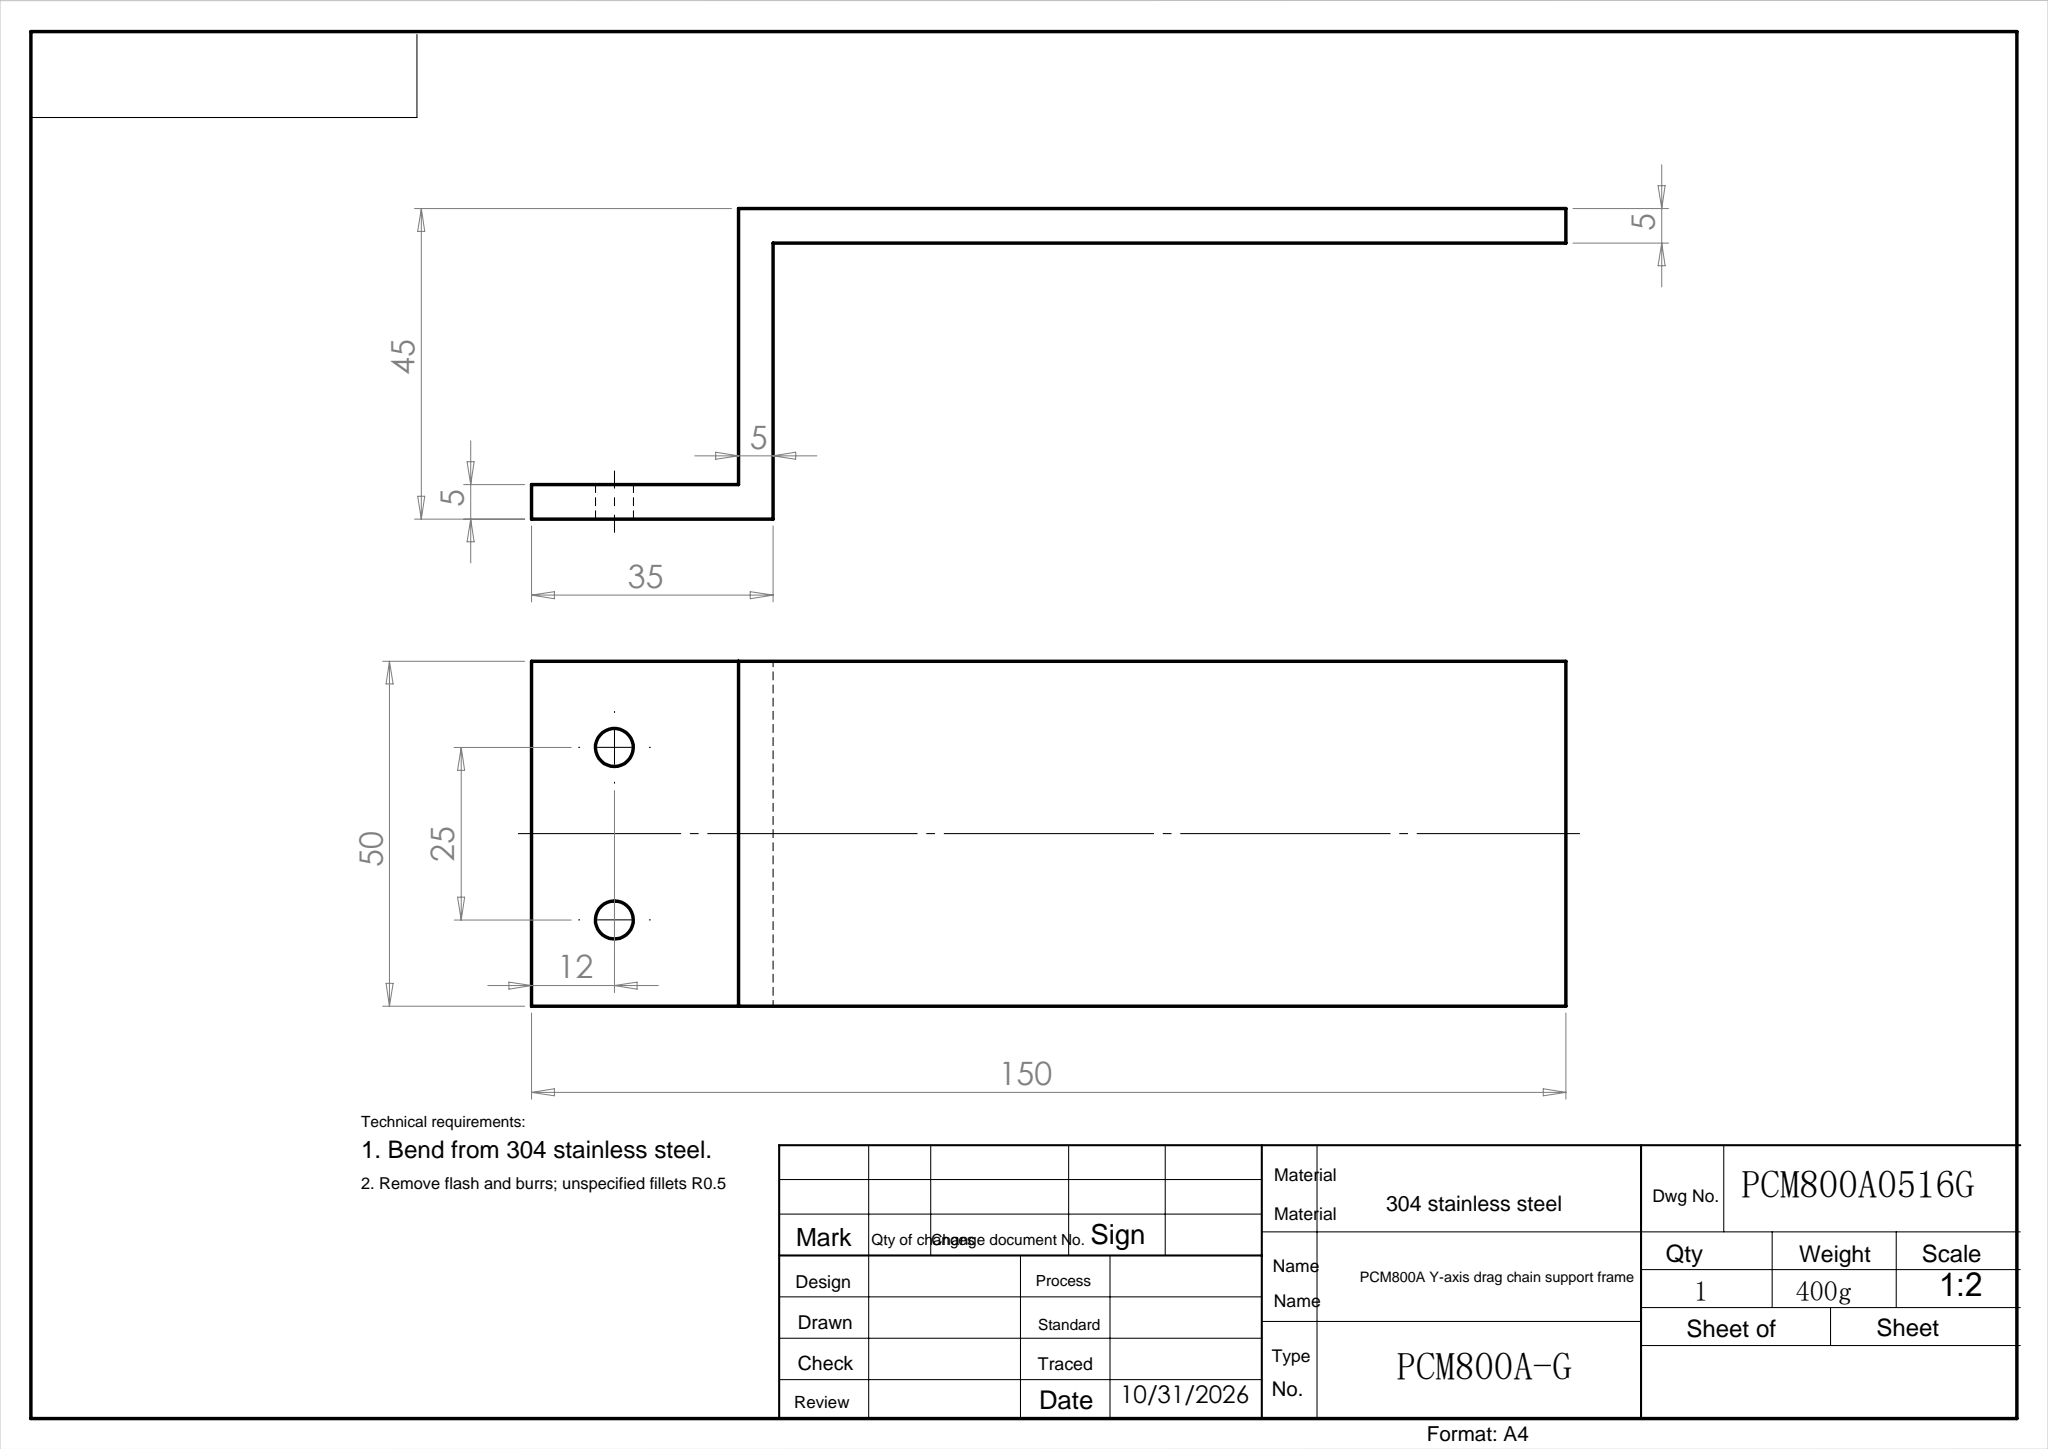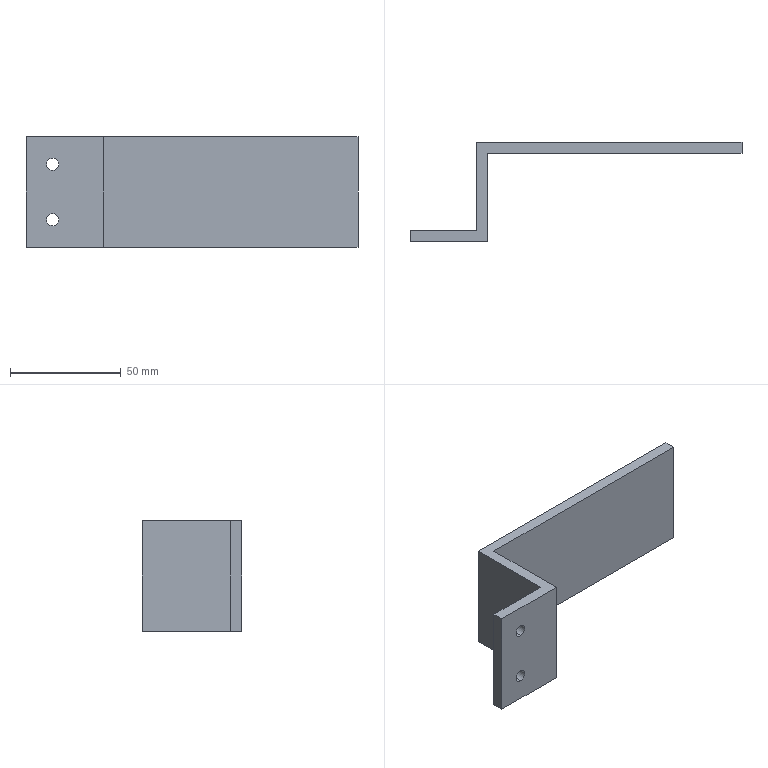Part | SolidWorks | features ExtruThin 1, ICE 1 | 1 solid | 14 faces | box 150 x 45 x 50 mm | volume 47262 mm3 | plane 10 | cylinder 4 | commonest cylinder face diameters 5.5 x4
STEP:
#1=CARTESIAN_POINT('',(12.,-5.,34.75));
#2=VERTEX_POINT('',#1);
#3=CARTESIAN_POINT('',(12.,-5.,40.25));
#4=VERTEX_POINT('',#3);
#5=CARTESIAN_POINT('',(12.,-5.,37.5));
#6=DIRECTION('',(0.,1.,0.));
#7=DIRECTION('',(0.,0.,1.));
#8=AXIS2_PLACEMENT_3D('',#5,#6,#7);
#9=CIRCLE('',#8,2.75);
#10=EDGE_CURVE('',#2,#4,#9,.T.);
#11=ORIENTED_EDGE('',*,*,#10,.F.);
#12=CARTESIAN_POINT('',(12.,0.,34.75));
#13=VERTEX_POINT('',#12);
#14=CARTESIAN_POINT('',(12.,-10.,34.75));
#15=DIRECTION('',(0.,1.,0.));
#16=VECTOR('',#15,1000.);
#17=LINE('',#14,#16);
#18=EDGE_CURVE('',#2,#13,#17,.T.);
#19=ORIENTED_EDGE('',*,*,#18,.T.);
#20=CARTESIAN_POINT('',(12.,0.,40.25));
#21=VERTEX_POINT('',#20);
#22=CARTESIAN_POINT('',(12.,0.,37.5));
#23=DIRECTION('',(0.,1.,0.));
#24=DIRECTION('',(0.,0.,-1.));
#25=AXIS2_PLACEMENT_3D('',#22,#23,#24);
#26=CIRCLE('',#25,2.75);
#27=EDGE_CURVE('',#13,#21,#26,.T.);
#28=ORIENTED_EDGE('',*,*,#27,.T.);
#29=CARTESIAN_POINT('',(12.,-10.,40.25));
#30=DIRECTION('',(0.,1.,0.));
#31=VECTOR('',#30,1000.);
#32=LINE('',#29,#31);
#33=EDGE_CURVE('',#4,#21,#32,.T.);
#34=ORIENTED_EDGE('',*,*,#33,.F.);
#35=EDGE_LOOP('',(#11,#19,#28,#34));
#36=FACE_OUTER_BOUND('',#35,.T.);
#37=CARTESIAN_POINT('',(12.,-10.,37.5));
#38=DIRECTION('',(0.,1.,0.));
#39=DIRECTION('',(0.,0.,1.));
#40=AXIS2_PLACEMENT_3D('',#37,#38,#39);
#41=CYLINDRICAL_SURFACE('',#40,2.75);
#42=ADVANCED_FACE('',(#36),#41,.F.);
#43=CARTESIAN_POINT('',(12.,-5.,9.75));
#44=VERTEX_POINT('',#43);
#45=CARTESIAN_POINT('',(12.,-5.,15.25));
#46=VERTEX_POINT('',#45);
#47=CARTESIAN_POINT('',(12.,-5.,12.5));
#48=DIRECTION('',(0.,1.,0.));
#49=DIRECTION('',(0.,0.,1.));
#50=AXIS2_PLACEMENT_3D('',#47,#48,#49);
#51=CIRCLE('',#50,2.75);
#52=EDGE_CURVE('',#44,#46,#51,.T.);
#53=ORIENTED_EDGE('',*,*,#52,.F.);
#54=CARTESIAN_POINT('',(12.,0.,9.75));
#55=VERTEX_POINT('',#54);
#56=CARTESIAN_POINT('',(12.,-10.,9.75));
#57=DIRECTION('',(0.,1.,0.));
#58=VECTOR('',#57,1000.);
#59=LINE('',#56,#58);
#60=EDGE_CURVE('',#44,#55,#59,.T.);
#61=ORIENTED_EDGE('',*,*,#60,.T.);
#62=CARTESIAN_POINT('',(12.,0.,15.25));
#63=VERTEX_POINT('',#62);
#64=CARTESIAN_POINT('',(12.,0.,12.5));
#65=DIRECTION('',(0.,1.,0.));
#66=DIRECTION('',(0.,0.,1.));
#67=AXIS2_PLACEMENT_3D('',#64,#65,#66);
#68=CIRCLE('',#67,2.75);
#69=EDGE_CURVE('',#55,#63,#68,.T.);
#70=ORIENTED_EDGE('',*,*,#69,.T.);
#71=CARTESIAN_POINT('',(12.,-10.,15.25));
#72=DIRECTION('',(0.,1.,0.));
#73=VECTOR('',#72,1000.);
#74=LINE('',#71,#73);
#75=EDGE_CURVE('',#46,#63,#74,.T.);
#76=ORIENTED_EDGE('',*,*,#75,.F.);
#77=EDGE_LOOP('',(#53,#61,#70,#76));
#78=FACE_OUTER_BOUND('',#77,.T.);
#79=CARTESIAN_POINT('',(12.,-10.,12.5));
#80=DIRECTION('',(0.,1.,0.));
#81=DIRECTION('',(0.,0.,1.));
#82=AXIS2_PLACEMENT_3D('',#79,#80,#81);
#83=CYLINDRICAL_SURFACE('',#82,2.75);
#84=ADVANCED_FACE('',(#78),#83,.F.);
#85=CARTESIAN_POINT('',(35.,35.,0.));
#86=VERTEX_POINT('',#85);
#87=CARTESIAN_POINT('',(150.,35.,0.));
#88=VERTEX_POINT('',#87);
#89=CARTESIAN_POINT('',(30.,35.,0.));
#90=DIRECTION('',(1.,0.,0.));
#91=VECTOR('',#90,1000.);
#92=LINE('',#89,#91);
#93=EDGE_CURVE('',#86,#88,#92,.T.);
#94=ORIENTED_EDGE('',*,*,#93,.T.);
#95=CARTESIAN_POINT('',(150.,35.,50.));
#96=VERTEX_POINT('',#95);
#97=CARTESIAN_POINT('',(150.,35.,50.));
#98=DIRECTION('',(0.,0.,-1.));
#99=VECTOR('',#98,1000.);
#100=LINE('',#97,#99);
#101=EDGE_CURVE('',#96,#88,#100,.T.);
#102=ORIENTED_EDGE('',*,*,#101,.F.);
#103=CARTESIAN_POINT('',(35.,35.,50.));
#104=VERTEX_POINT('',#103);
#105=CARTESIAN_POINT('',(30.,35.,50.));
#106=DIRECTION('',(1.,0.,0.));
#107=VECTOR('',#106,1000.);
#108=LINE('',#105,#107);
#109=EDGE_CURVE('',#104,#96,#108,.T.);
#110=ORIENTED_EDGE('',*,*,#109,.F.);
#111=CARTESIAN_POINT('',(35.,35.,50.));
#112=DIRECTION('',(0.,0.,-1.));
#113=VECTOR('',#112,1000.);
#114=LINE('',#111,#113);
#115=EDGE_CURVE('',#104,#86,#114,.T.);
#116=ORIENTED_EDGE('',*,*,#115,.T.);
#117=EDGE_LOOP('',(#94,#102,#110,#116));
#118=FACE_OUTER_BOUND('',#117,.T.);
#119=CARTESIAN_POINT('',(30.,35.,50.));
#120=DIRECTION('',(0.,1.,0.));
#121=DIRECTION('',(0.,0.,1.));
#122=AXIS2_PLACEMENT_3D('',#119,#120,#121);
#123=PLANE('',#122);
#124=ADVANCED_FACE('',(#118),#123,.F.);
#125=CARTESIAN_POINT('',(150.,40.,0.));
#126=VERTEX_POINT('',#125);
#127=CARTESIAN_POINT('',(150.,40.,0.));
#128=DIRECTION('',(0.,-1.,0.));
#129=VECTOR('',#128,1000.);
#130=LINE('',#127,#129);
#131=EDGE_CURVE('',#126,#88,#130,.T.);
#132=ORIENTED_EDGE('',*,*,#131,.F.);
#133=CARTESIAN_POINT('',(150.,40.,50.));
#134=VERTEX_POINT('',#133);
#135=CARTESIAN_POINT('',(150.,40.,50.));
#136=DIRECTION('',(0.,0.,-1.));
#137=VECTOR('',#136,1000.);
#138=LINE('',#135,#137);
#139=EDGE_CURVE('',#134,#126,#138,.T.);
#140=ORIENTED_EDGE('',*,*,#139,.F.);
#141=CARTESIAN_POINT('',(150.,40.,50.));
#142=DIRECTION('',(0.,-1.,0.));
#143=VECTOR('',#142,1000.);
#144=LINE('',#141,#143);
#145=EDGE_CURVE('',#134,#96,#144,.T.);
#146=ORIENTED_EDGE('',*,*,#145,.T.);
#147=ORIENTED_EDGE('',*,*,#101,.T.);
#148=EDGE_LOOP('',(#132,#140,#146,#147));
#149=FACE_OUTER_BOUND('',#148,.T.);
#150=CARTESIAN_POINT('',(150.,40.,50.));
#151=DIRECTION('',(1.,0.,0.));
#152=DIRECTION('',(0.,0.,-1.));
#153=AXIS2_PLACEMENT_3D('',#150,#151,#152);
#154=PLANE('',#153);
#155=ADVANCED_FACE('',(#149),#154,.T.);
#156=CARTESIAN_POINT('',(30.,40.,0.));
#157=VERTEX_POINT('',#156);
#158=CARTESIAN_POINT('',(30.,40.,0.));
#159=DIRECTION('',(1.,0.,0.));
#160=VECTOR('',#159,1000.);
#161=LINE('',#158,#160);
#162=EDGE_CURVE('',#157,#126,#161,.T.);
#163=ORIENTED_EDGE('',*,*,#162,.F.);
#164=CARTESIAN_POINT('',(30.,40.,50.));
#165=VERTEX_POINT('',#164);
#166=CARTESIAN_POINT('',(30.,40.,50.));
#167=DIRECTION('',(0.,0.,-1.));
#168=VECTOR('',#167,1000.);
#169=LINE('',#166,#168);
#170=EDGE_CURVE('',#165,#157,#169,.T.);
#171=ORIENTED_EDGE('',*,*,#170,.F.);
#172=CARTESIAN_POINT('',(30.,40.,50.));
#173=DIRECTION('',(1.,0.,0.));
#174=VECTOR('',#173,1000.);
#175=LINE('',#172,#174);
#176=EDGE_CURVE('',#165,#134,#175,.T.);
#177=ORIENTED_EDGE('',*,*,#176,.T.);
#178=ORIENTED_EDGE('',*,*,#139,.T.);
#179=EDGE_LOOP('',(#163,#171,#177,#178));
#180=FACE_OUTER_BOUND('',#179,.T.);
#181=CARTESIAN_POINT('',(30.,40.,50.));
#182=DIRECTION('',(0.,1.,0.));
#183=DIRECTION('',(0.,0.,1.));
#184=AXIS2_PLACEMENT_3D('',#181,#182,#183);
#185=PLANE('',#184);
#186=ADVANCED_FACE('',(#180),#185,.T.);
#187=CARTESIAN_POINT('',(30.,0.,0.));
#188=VERTEX_POINT('',#187);
#189=CARTESIAN_POINT('',(30.,0.,0.));
#190=DIRECTION('',(0.,1.,0.));
#191=VECTOR('',#190,1000.);
#192=LINE('',#189,#191);
#193=EDGE_CURVE('',#188,#157,#192,.T.);
#194=ORIENTED_EDGE('',*,*,#193,.F.);
#195=CARTESIAN_POINT('',(30.,0.,50.));
#196=VERTEX_POINT('',#195);
#197=CARTESIAN_POINT('',(30.,0.,50.));
#198=DIRECTION('',(0.,0.,-1.));
#199=VECTOR('',#198,1000.);
#200=LINE('',#197,#199);
#201=EDGE_CURVE('',#196,#188,#200,.T.);
#202=ORIENTED_EDGE('',*,*,#201,.F.);
#203=CARTESIAN_POINT('',(30.,0.,50.));
#204=DIRECTION('',(0.,1.,0.));
#205=VECTOR('',#204,1000.);
#206=LINE('',#203,#205);
#207=EDGE_CURVE('',#196,#165,#206,.T.);
#208=ORIENTED_EDGE('',*,*,#207,.T.);
#209=ORIENTED_EDGE('',*,*,#170,.T.);
#210=EDGE_LOOP('',(#194,#202,#208,#209));
#211=FACE_OUTER_BOUND('',#210,.T.);
#212=CARTESIAN_POINT('',(30.,0.,50.));
#213=DIRECTION('',(-1.,0.,0.));
#214=DIRECTION('',(0.,0.,1.));
#215=AXIS2_PLACEMENT_3D('',#212,#213,#214);
#216=PLANE('',#215);
#217=ADVANCED_FACE('',(#211),#216,.T.);
#218=CARTESIAN_POINT('',(12.,0.,37.5));
#219=DIRECTION('',(0.,1.,0.));
#220=DIRECTION('',(0.,0.,-1.));
#221=AXIS2_PLACEMENT_3D('',#218,#219,#220);
#222=CIRCLE('',#221,2.75);
#223=EDGE_CURVE('',#21,#13,#222,.T.);
#224=ORIENTED_EDGE('',*,*,#223,.F.);
#225=ORIENTED_EDGE('',*,*,#27,.F.);
#226=EDGE_LOOP('',(#224,#225));
#227=FACE_BOUND('',#226,.T.);
#228=CARTESIAN_POINT('',(12.,0.,12.5));
#229=DIRECTION('',(0.,1.,0.));
#230=DIRECTION('',(0.,0.,1.));
#231=AXIS2_PLACEMENT_3D('',#228,#229,#230);
#232=CIRCLE('',#231,2.75);
#233=EDGE_CURVE('',#63,#55,#232,.T.);
#234=ORIENTED_EDGE('',*,*,#233,.F.);
#235=ORIENTED_EDGE('',*,*,#69,.F.);
#236=EDGE_LOOP('',(#234,#235));
#237=FACE_BOUND('',#236,.T.);
#238=CARTESIAN_POINT('',(0.,0.,0.));
#239=VERTEX_POINT('',#238);
#240=CARTESIAN_POINT('',(0.,0.,0.));
#241=DIRECTION('',(1.,0.,0.));
#242=VECTOR('',#241,1000.);
#243=LINE('',#240,#242);
#244=EDGE_CURVE('',#239,#188,#243,.T.);
#245=ORIENTED_EDGE('',*,*,#244,.F.);
#246=CARTESIAN_POINT('',(0.,0.,50.));
#247=VERTEX_POINT('',#246);
#248=CARTESIAN_POINT('',(0.,0.,50.));
#249=DIRECTION('',(0.,0.,-1.));
#250=VECTOR('',#249,1000.);
#251=LINE('',#248,#250);
#252=EDGE_CURVE('',#247,#239,#251,.T.);
#253=ORIENTED_EDGE('',*,*,#252,.F.);
#254=CARTESIAN_POINT('',(0.,0.,50.));
#255=DIRECTION('',(1.,0.,0.));
#256=VECTOR('',#255,1000.);
#257=LINE('',#254,#256);
#258=EDGE_CURVE('',#247,#196,#257,.T.);
#259=ORIENTED_EDGE('',*,*,#258,.T.);
#260=ORIENTED_EDGE('',*,*,#201,.T.);
#261=EDGE_LOOP('',(#245,#253,#259,#260));
#262=FACE_OUTER_BOUND('',#261,.T.);
#263=CARTESIAN_POINT('',(0.,0.,50.));
#264=DIRECTION('',(0.,1.,0.));
#265=DIRECTION('',(0.,0.,1.));
#266=AXIS2_PLACEMENT_3D('',#263,#264,#265);
#267=PLANE('',#266);
#268=ADVANCED_FACE('',(#227,#237,#262),#267,.T.);
#269=CARTESIAN_POINT('',(0.,-5.,0.));
#270=VERTEX_POINT('',#269);
#271=CARTESIAN_POINT('',(0.,-5.,0.));
#272=DIRECTION('',(0.,1.,0.));
#273=VECTOR('',#272,1000.);
#274=LINE('',#271,#273);
#275=EDGE_CURVE('',#270,#239,#274,.T.);
#276=ORIENTED_EDGE('',*,*,#275,.F.);
#277=CARTESIAN_POINT('',(0.,-5.,50.));
#278=VERTEX_POINT('',#277);
#279=CARTESIAN_POINT('',(0.,-5.,50.));
#280=DIRECTION('',(0.,0.,-1.));
#281=VECTOR('',#280,1000.);
#282=LINE('',#279,#281);
#283=EDGE_CURVE('',#278,#270,#282,.T.);
#284=ORIENTED_EDGE('',*,*,#283,.F.);
#285=CARTESIAN_POINT('',(0.,-5.,50.));
#286=DIRECTION('',(0.,1.,0.));
#287=VECTOR('',#286,1000.);
#288=LINE('',#285,#287);
#289=EDGE_CURVE('',#278,#247,#288,.T.);
#290=ORIENTED_EDGE('',*,*,#289,.T.);
#291=ORIENTED_EDGE('',*,*,#252,.T.);
#292=EDGE_LOOP('',(#276,#284,#290,#291));
#293=FACE_OUTER_BOUND('',#292,.T.);
#294=CARTESIAN_POINT('',(0.,-5.,50.));
#295=DIRECTION('',(-1.,0.,0.));
#296=DIRECTION('',(0.,0.,1.));
#297=AXIS2_PLACEMENT_3D('',#294,#295,#296);
#298=PLANE('',#297);
#299=ADVANCED_FACE('',(#293),#298,.T.);
#300=CARTESIAN_POINT('',(12.,-5.,37.5));
#301=DIRECTION('',(0.,1.,0.));
#302=DIRECTION('',(0.,0.,1.));
#303=AXIS2_PLACEMENT_3D('',#300,#301,#302);
#304=CIRCLE('',#303,2.75);
#305=EDGE_CURVE('',#4,#2,#304,.T.);
#306=ORIENTED_EDGE('',*,*,#305,.T.);
#307=ORIENTED_EDGE('',*,*,#10,.T.);
#308=EDGE_LOOP('',(#306,#307));
#309=FACE_BOUND('',#308,.T.);
#310=CARTESIAN_POINT('',(12.,-5.,12.5));
#311=DIRECTION('',(0.,1.,0.));
#312=DIRECTION('',(0.,0.,1.));
#313=AXIS2_PLACEMENT_3D('',#310,#311,#312);
#314=CIRCLE('',#313,2.75);
#315=EDGE_CURVE('',#46,#44,#314,.T.);
#316=ORIENTED_EDGE('',*,*,#315,.T.);
#317=ORIENTED_EDGE('',*,*,#52,.T.);
#318=EDGE_LOOP('',(#316,#317));
#319=FACE_BOUND('',#318,.T.);
#320=CARTESIAN_POINT('',(35.,-5.,0.));
#321=VERTEX_POINT('',#320);
#322=CARTESIAN_POINT('',(0.,-5.,0.));
#323=DIRECTION('',(1.,0.,0.));
#324=VECTOR('',#323,1000.);
#325=LINE('',#322,#324);
#326=EDGE_CURVE('',#270,#321,#325,.T.);
#327=ORIENTED_EDGE('',*,*,#326,.T.);
#328=CARTESIAN_POINT('',(35.,-5.,50.));
#329=VERTEX_POINT('',#328);
#330=CARTESIAN_POINT('',(35.,-5.,50.));
#331=DIRECTION('',(0.,0.,-1.));
#332=VECTOR('',#331,1000.);
#333=LINE('',#330,#332);
#334=EDGE_CURVE('',#329,#321,#333,.T.);
#335=ORIENTED_EDGE('',*,*,#334,.F.);
#336=CARTESIAN_POINT('',(0.,-5.,50.));
#337=DIRECTION('',(1.,0.,0.));
#338=VECTOR('',#337,1000.);
#339=LINE('',#336,#338);
#340=EDGE_CURVE('',#278,#329,#339,.T.);
#341=ORIENTED_EDGE('',*,*,#340,.F.);
#342=ORIENTED_EDGE('',*,*,#283,.T.);
#343=EDGE_LOOP('',(#327,#335,#341,#342));
#344=FACE_OUTER_BOUND('',#343,.T.);
#345=CARTESIAN_POINT('',(0.,-5.,50.));
#346=DIRECTION('',(0.,1.,0.));
#347=DIRECTION('',(0.,0.,1.));
#348=AXIS2_PLACEMENT_3D('',#345,#346,#347);
#349=PLANE('',#348);
#350=ADVANCED_FACE('',(#309,#319,#344),#349,.F.);
#351=CARTESIAN_POINT('',(35.,0.,0.));
#352=DIRECTION('',(0.,1.,0.));
#353=VECTOR('',#352,1000.);
#354=LINE('',#351,#353);
#355=EDGE_CURVE('',#321,#86,#354,.T.);
#356=ORIENTED_EDGE('',*,*,#355,.T.);
#357=ORIENTED_EDGE('',*,*,#115,.F.);
#358=CARTESIAN_POINT('',(35.,0.,50.));
#359=DIRECTION('',(0.,1.,0.));
#360=VECTOR('',#359,1000.);
#361=LINE('',#358,#360);
#362=EDGE_CURVE('',#329,#104,#361,.T.);
#363=ORIENTED_EDGE('',*,*,#362,.F.);
#364=ORIENTED_EDGE('',*,*,#334,.T.);
#365=EDGE_LOOP('',(#356,#357,#363,#364));
#366=FACE_OUTER_BOUND('',#365,.T.);
#367=CARTESIAN_POINT('',(35.,0.,50.));
#368=DIRECTION('',(-1.,0.,0.));
#369=DIRECTION('',(0.,0.,1.));
#370=AXIS2_PLACEMENT_3D('',#367,#368,#369);
#371=PLANE('',#370);
#372=ADVANCED_FACE('',(#366),#371,.F.);
#373=ORIENTED_EDGE('',*,*,#109,.T.);
#374=ORIENTED_EDGE('',*,*,#145,.F.);
#375=ORIENTED_EDGE('',*,*,#176,.F.);
#376=ORIENTED_EDGE('',*,*,#207,.F.);
#377=ORIENTED_EDGE('',*,*,#258,.F.);
#378=ORIENTED_EDGE('',*,*,#289,.F.);
#379=ORIENTED_EDGE('',*,*,#340,.T.);
#380=ORIENTED_EDGE('',*,*,#362,.T.);
#381=EDGE_LOOP('',(#373,#374,#375,#376,#377,#378,#379,#380));
#382=FACE_OUTER_BOUND('',#381,.T.);
#383=CARTESIAN_POINT('',(150.,35.,50.));
#384=DIRECTION('',(0.,0.,-1.));
#385=DIRECTION('',(-1.,0.,0.));
#386=AXIS2_PLACEMENT_3D('',#383,#384,#385);
#387=PLANE('',#386);
#388=ADVANCED_FACE('',(#382),#387,.F.);
#389=ORIENTED_EDGE('',*,*,#93,.F.);
#390=ORIENTED_EDGE('',*,*,#355,.F.);
#391=ORIENTED_EDGE('',*,*,#326,.F.);
#392=ORIENTED_EDGE('',*,*,#275,.T.);
#393=ORIENTED_EDGE('',*,*,#244,.T.);
#394=ORIENTED_EDGE('',*,*,#193,.T.);
#395=ORIENTED_EDGE('',*,*,#162,.T.);
#396=ORIENTED_EDGE('',*,*,#131,.T.);
#397=EDGE_LOOP('',(#389,#390,#391,#392,#393,#394,#395,#396));
#398=FACE_OUTER_BOUND('',#397,.T.);
#399=CARTESIAN_POINT('',(150.,35.,0.));
#400=DIRECTION('',(0.,0.,-1.));
#401=DIRECTION('',(-1.,0.,0.));
#402=AXIS2_PLACEMENT_3D('',#399,#400,#401);
#403=PLANE('',#402);
#404=ADVANCED_FACE('',(#398),#403,.T.);
#405=ORIENTED_EDGE('',*,*,#60,.F.);
#406=ORIENTED_EDGE('',*,*,#315,.F.);
#407=ORIENTED_EDGE('',*,*,#75,.T.);
#408=ORIENTED_EDGE('',*,*,#233,.T.);
#409=EDGE_LOOP('',(#405,#406,#407,#408));
#410=FACE_OUTER_BOUND('',#409,.T.);
#411=CARTESIAN_POINT('',(12.,-10.,12.5));
#412=DIRECTION('',(0.,1.,0.));
#413=DIRECTION('',(0.,0.,1.));
#414=AXIS2_PLACEMENT_3D('',#411,#412,#413);
#415=CYLINDRICAL_SURFACE('',#414,2.75);
#416=ADVANCED_FACE('',(#410),#415,.F.);
#417=ORIENTED_EDGE('',*,*,#18,.F.);
#418=ORIENTED_EDGE('',*,*,#305,.F.);
#419=ORIENTED_EDGE('',*,*,#33,.T.);
#420=ORIENTED_EDGE('',*,*,#223,.T.);
#421=EDGE_LOOP('',(#417,#418,#419,#420));
#422=FACE_OUTER_BOUND('',#421,.T.);
#423=CARTESIAN_POINT('',(12.,-10.,37.5));
#424=DIRECTION('',(0.,1.,0.));
#425=DIRECTION('',(0.,0.,1.));
#426=AXIS2_PLACEMENT_3D('',#423,#424,#425);
#427=CYLINDRICAL_SURFACE('',#426,2.75);
#428=ADVANCED_FACE('',(#422),#427,.F.);
#429=CLOSED_SHELL('',(#42,#84,#124,#155,#186,#217,#268,#299,#350,#372,#388,#404,#416,#428));
#430=MANIFOLD_SOLID_BREP('',#429);
#431=CARTESIAN_POINT('',(0.,0.,0.));
#432=DIRECTION('',(0.,0.,1.));
#433=DIRECTION('',(1.,0.,0.));
#434=AXIS2_PLACEMENT_3D('',#431,#432,#433);
#435=(LENGTH_UNIT()NAMED_UNIT(*)SI_UNIT(.MILLI.,.METRE.));
#436=UNCERTAINTY_MEASURE_WITH_UNIT(LENGTH_MEASURE(0.00001),#435,'','');
#437=(NAMED_UNIT(*)PLANE_ANGLE_UNIT()SI_UNIT($,.RADIAN.));
#438=(NAMED_UNIT(*)SI_UNIT($,.STERADIAN.)SOLID_ANGLE_UNIT());
#439=(GEOMETRIC_REPRESENTATION_CONTEXT(3)GLOBAL_UNCERTAINTY_ASSIGNED_CONTEXT((#436))GLOBAL_UNIT_ASSIGNED_CONTEXT((#435,#437,#438))REPRESENTATION_CONTEXT('',''));
#440=ADVANCED_BREP_SHAPE_REPRESENTATION('',(#430,#434),#439);